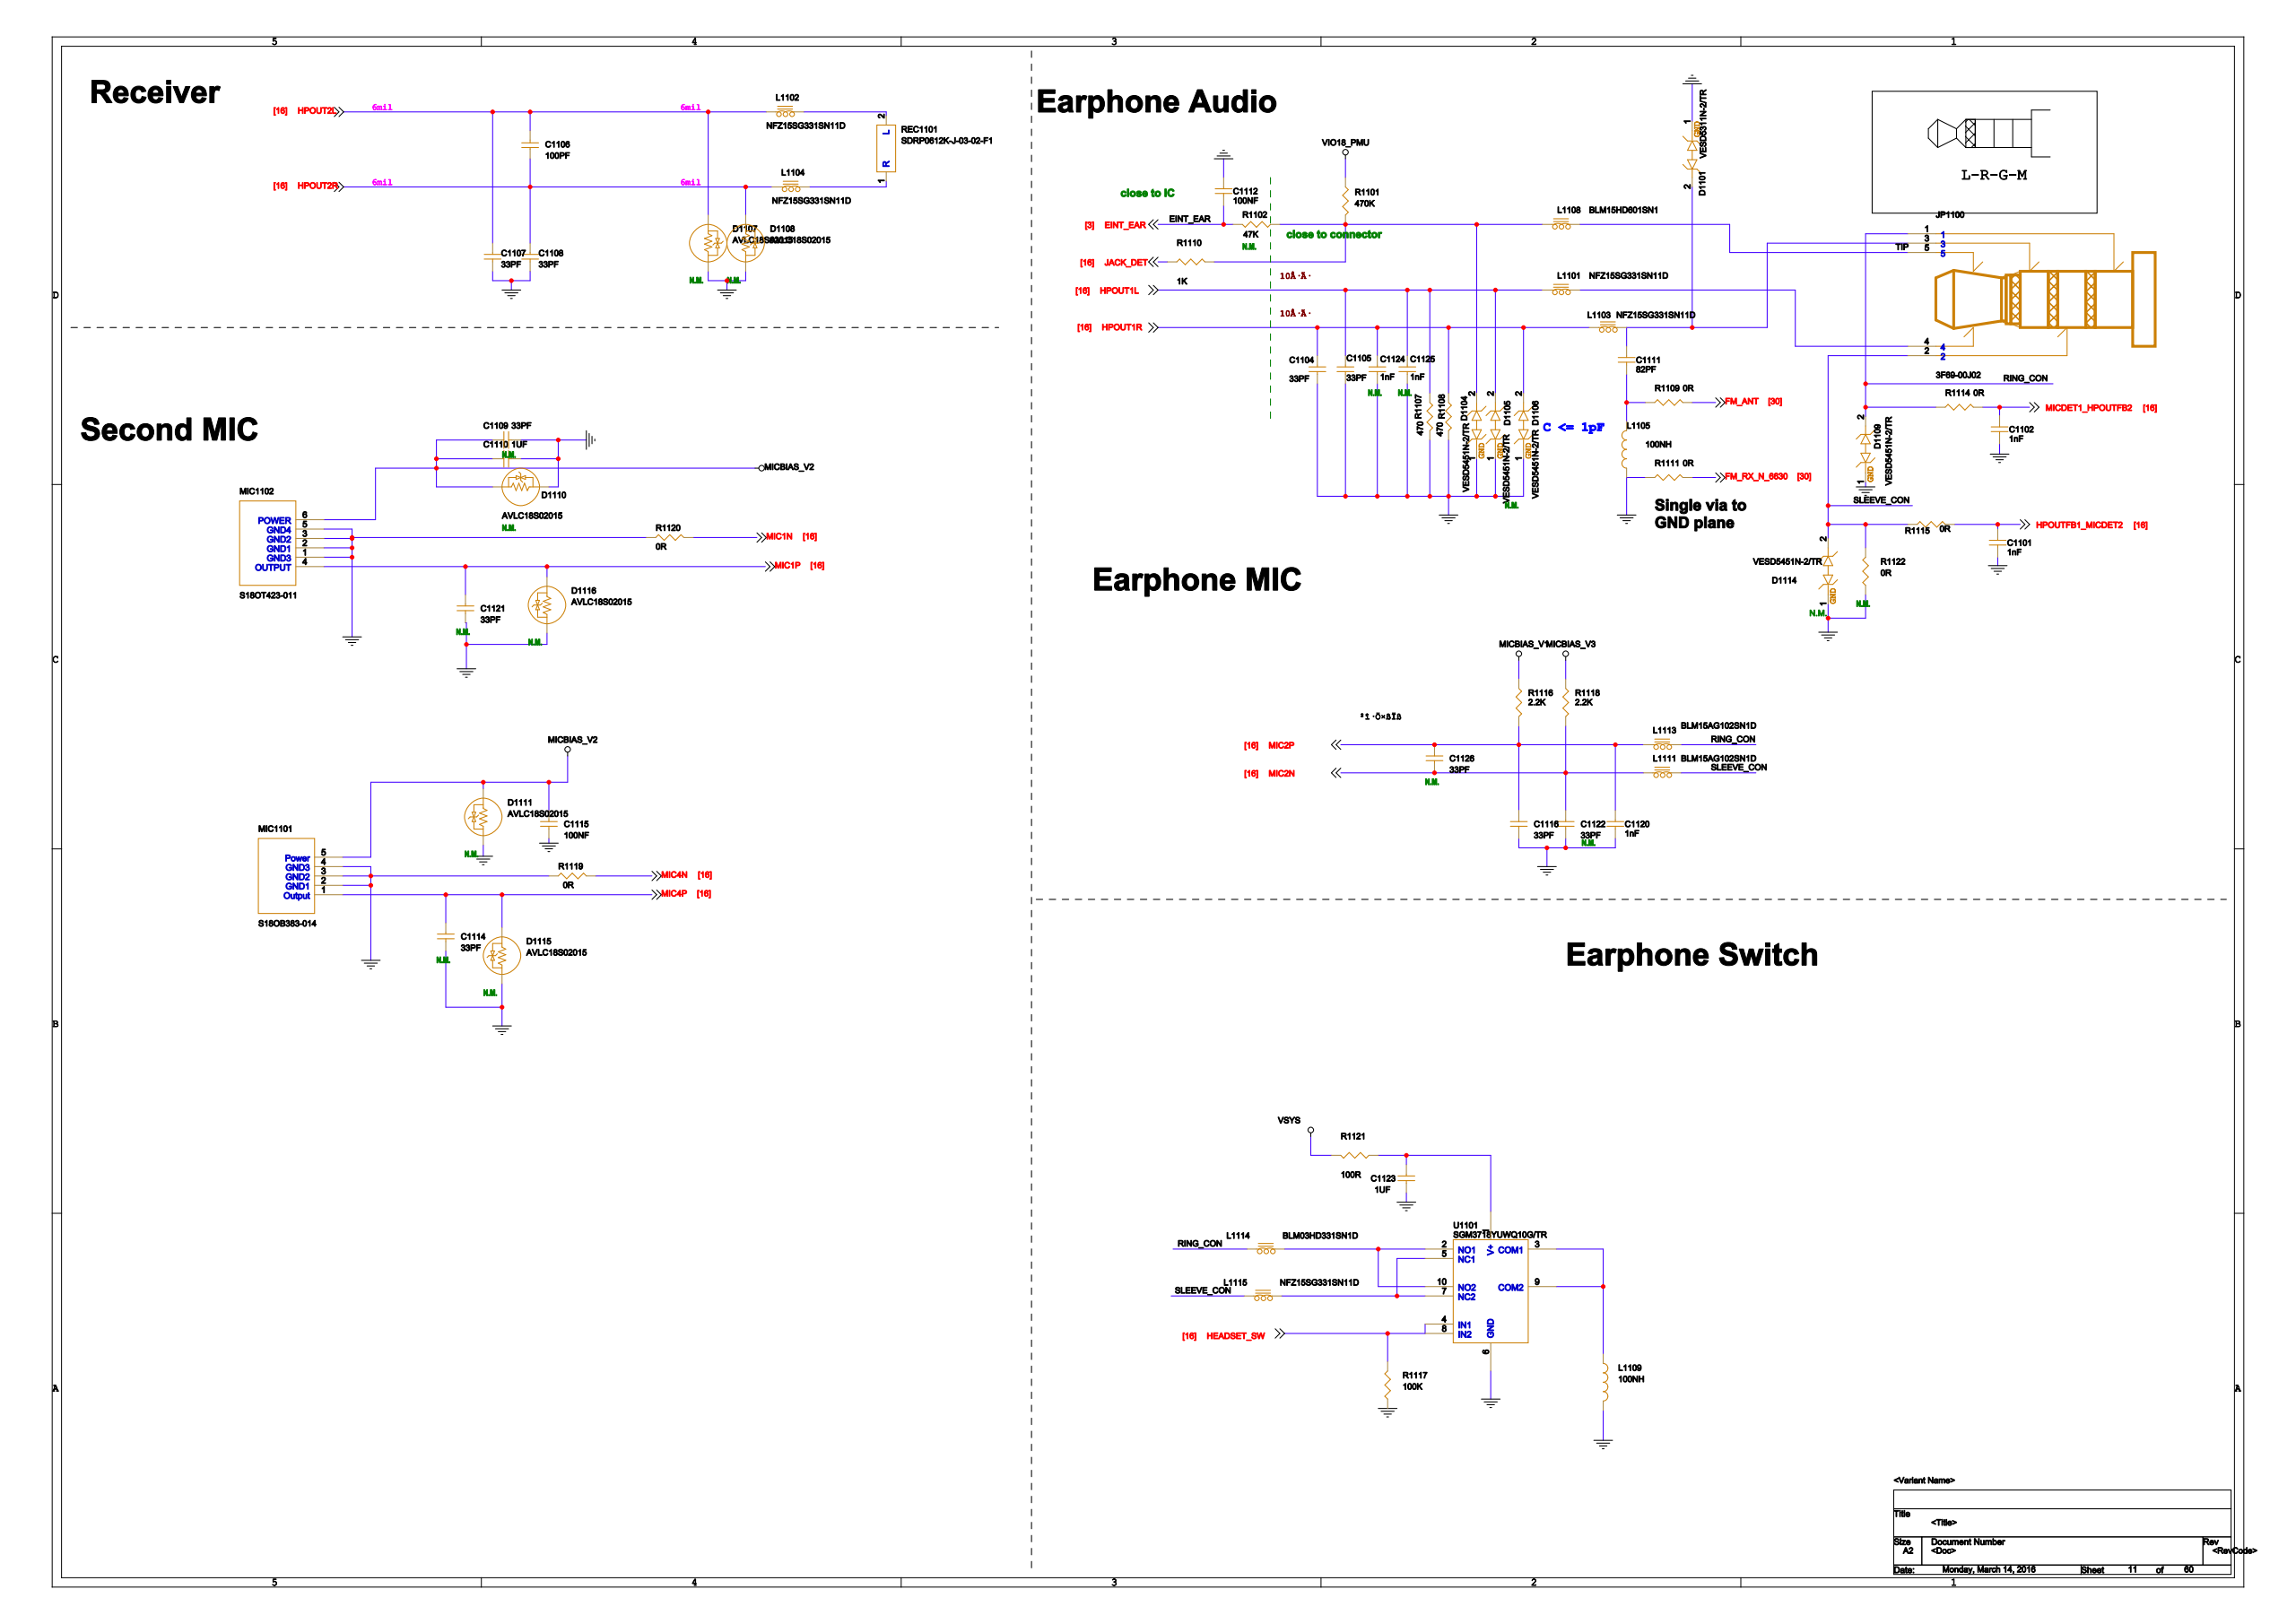Circuit board | Cadence Allegro | 1088 parts | 793 nets | one sheet of the schematic
Parts on this sheet (reference | value | footprint):
C1101 | 1nF | C0201
C1102 | 1nF | C0201
C1104 | 33PF | C0201
C1105 | 33PF | C0201
C1106 | 100PF | C0201
C1107 | 33PF | C0201
C1108 | 33PF | C0201
C1109
C1110 | 1UF | C0201
C1111 | 82PF | C0201
C1112 | 100NF | C0201
C1114
C1115 | 100NF | C0201
C1116 | 33PF | C0201
C1120 | 1nF | C0201
C1121
C1122
C1123 | 1UF | C0201
C1124
C1125
C1126
D1101 | VESD5311N-2/TR | DFN1006-2
D1104 | VESD5451N-2/TR | DFN1006-2
D1105 | VESD5451N-2/TR | DFN1006-2
D1106
D1107
D1108
D1109 | VESD5451N-2/TR | DFN1006-2
D1110
D1111
D1114
D1115
D1116
JP1100 | 3F69-00J02 | HP_3F69-00J02
L1101 | NFZ15SG331SN11D | L0402
L1102 | NFZ15SG331SN11D | L0402
L1103 | NFZ15SG331SN11D | L0402
L1104 | NFZ15SG331SN11D | L0402
L1105 | 100NH | L0603
L1108 | BLM15HD601SN1 | L0402
L1109 | 100NH | L0603
L1111 | BLM15AG102SN1D | L0402
L1113 | BLM15AG102SN1D | L0402
L1114 | BLM03HD331SN1D | FB0201
L1115 | NFZ15SG331SN11D | L0402
MIC1101 | S18OB383-014 | S18OB383-014
MIC1102 | S18OT423-011 | MIC_S18OT381-012
R1101 | 470K | R0201
R1102
R1107 | 470 | R0201
R1108 | 470 | R0201
R1109 | 0R | R0201
R1110 | 1K | R0201
R1111 | 0R | R0201
R1114 | 0R | R0201
R1115 | 0R | R0201
R1116 | 2.2K | R0201
R1117 | 100K | R0201
R1118 | 2.2K | R0201
R1119 | 0R | R0201
R1120 | 0R | R0201
R1121 | 100R | R0201
R1122
REC1101 | SDRP0612K-J-03-02-F1 | REC_SDRP0612K-J-03-02-F1
U1101 | SGM3718YUWQ10G/TR | TQFN10_1P4X1P8X0P9_0P4
Nets of these parts (net: part-pin ...):
RING_CON: D1109-2 JP1100-1 L1113-2 L1114-1 R1114-1
N33529224: L1114-2 U1101-2 U1101-10
GND: C1101-2 C1102-2 C1104-2 C1105-2 C1107-2 C1108-2 C1109-2 C1110-2 C1112-1 C1114-2 C1115-2 C1116-2 C1120-2 C1121-2 C1122-2 C1123-2 C1124-2 C1125-2 D1101-1 D1104-1 D1105-1 D1106-1 D1107-2 D1108-2 D1109-1 D1110-2 D1111-1 D1114-1 D1115-1 D1116-1 L1105-1 L1109-2 MIC1101-2 MIC1101-3 MIC1101-4 MIC1102-1 MIC1102-2 MIC1102-3 MIC1102-5 R1107-2 R1108-2 R1111-1 R1117-1 R1119-1 R1120-1 R1122-1 U1101-6
VSYS: R1121-2
MIC4P: C1114-1 D1115-2 MIC1101-1
MICBIAS_V2: C1109-1 C1110-1 C1115-1 D1110-1 D1111-2 MIC1101-5 MIC1102-6
MIC1P: C1121-1 D1116-2 MIC1102-4
EINT_EAR: C1112-2 R1102-2
VIO18_PMU: R1101-1
HPOUT2L: C1106-2 C1107-1 D1107-1 L1102-1
HPOUT2R: C1106-1 C1108-1 D1108-1 L1104-1
SLEEVE_CON: D1114-2 JP1100-2 L1111-2 L1115-1 R1115-1 R1122-2
N33529233: L1115-2 U1101-5 U1101-7
N34856628: L1102-2 REC1101-2
N34856642: L1104-2 REC1101-1
HPOUT1L: C1105-1 C1125-1 D1105-2 L1101-1 R1107-1
N18434303: JP1100-4 L1101-2
HPOUT1R: C1104-1 C1124-1 D1106-2 L1103-1 R1108-1
N18434282: C1111-1 D1101-2 JP1100-3 L1103-2
TIP: JP1100-5 L1108-2
HEADSET_SW: R1117-2 U1101-4 U1101-8
HPOUTFB1_MICDET2: C1101-1 R1115-2
JACK_DET: R1110-1
MICDET1_HPOUTFB2: C1102-1 R1114-2
MICBIAS_V1: R1116-1
MICBIAS_V3: R1118-1
FM_RX_N_6630: R1111-2
N20113364: D1104-2 L1108-1 R1101-2 R1102-1 R1110-2
N33529266: C1123-1 R1121-1 U1101-1
MIC1N: R1120-2
MIC2P: C1116-1 C1120-1 C1126-1 L1113-1 R1116-2
MIC2N: C1122-1 C1126-2 L1111-1 R1118-2
MIC4N: R1119-2
N18451095: C1111-2 L1105-2 R1109-1
N33529243: L1109-1 U1101-3 U1101-9
FM_ANT: R1109-2